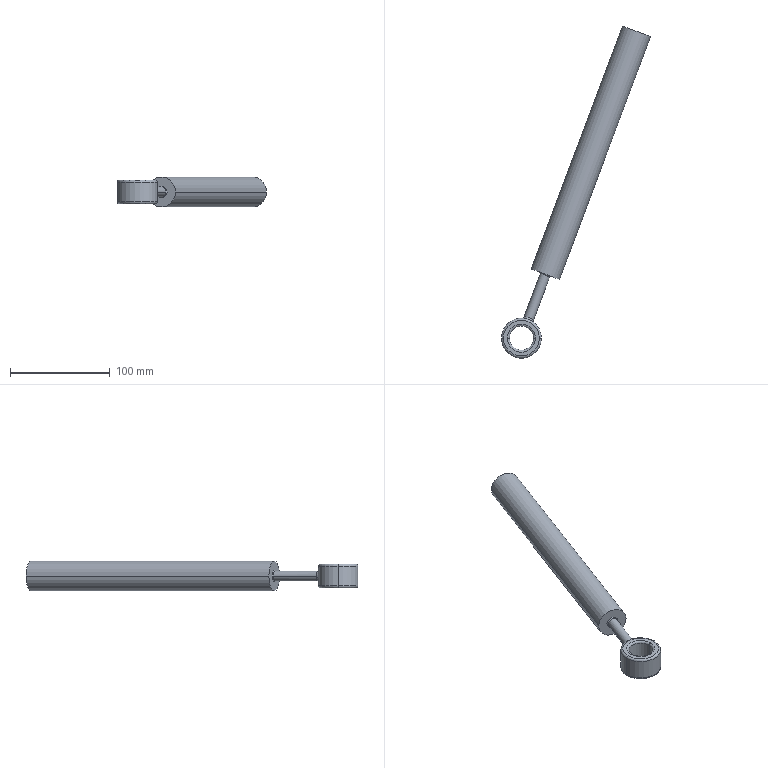Part | SolidWorks | features Fillet 2, ICE 2, Chamfer 1, Extrusion 1 | 1 solid | 24 faces | box 149.428 x 332.875 x 30.111 mm | volume 207967 mm3 | torus 8 | cylinder 8 | plane 4 | cone 2 | spline 2 | commonest cylinder face diameters 10 x2 24 x2 30.111 x2 40 x2
STEP:
#1=CARTESIAN_POINT('',(599.329,28.443,2335.07));
#2=VERTEX_POINT('',#1);
#3=CARTESIAN_POINT('',(589.965,31.954,2335.07));
#4=VERTEX_POINT('',#3);
#5=CARTESIAN_POINT('',(594.647,30.198,2335.07));
#6=DIRECTION('',(-0.3511,-0.9363,0.));
#7=DIRECTION('',(0.9363,-0.3511,0.));
#8=AXIS2_PLACEMENT_3D('',#5,#6,#7);
#9=CIRCLE('',#8,5.);
#10=EDGE_CURVE('',#2,#4,#9,.T.);
#11=ORIENTED_EDGE('',*,*,#10,.F.);
#12=CARTESIAN_POINT('',(600.616,29.028,2335.07));
#13=VERTEX_POINT('',#12);
#14=CARTESIAN_POINT('',(599.329,28.443,2335.07));
#15=DIRECTION('',(0.9103,0.4138,0.));
#16=VECTOR('',#15,1000.);
#17=LINE('',#14,#16);
#18=EDGE_CURVE('',#2,#13,#17,.T.);
#19=ORIENTED_EDGE('',*,*,#18,.T.);
#20=CARTESIAN_POINT('',(589.38,33.241,2335.07));
#21=VERTEX_POINT('',#20);
#22=CARTESIAN_POINT('',(594.998,31.135,2335.07));
#23=DIRECTION('',(0.3511,0.9363,0.));
#24=DIRECTION('',(0.9363,-0.3511,0.));
#25=AXIS2_PLACEMENT_3D('',#22,#23,#24);
#26=CIRCLE('',#25,6.);
#27=EDGE_CURVE('',#21,#13,#26,.T.);
#28=ORIENTED_EDGE('',*,*,#27,.F.);
#29=CARTESIAN_POINT('',(589.965,31.954,2335.07));
#30=DIRECTION('',(-0.4138,0.9103,0.));
#31=VECTOR('',#30,1000.);
#32=LINE('',#29,#31);
#33=EDGE_CURVE('',#4,#21,#32,.T.);
#34=ORIENTED_EDGE('',*,*,#33,.F.);
#35=EDGE_LOOP('',(#11,#19,#28,#34));
#36=FACE_OUTER_BOUND('',#35,.T.);
#37=CARTESIAN_POINT('',(594.647,30.198,2335.07));
#38=DIRECTION('',(0.3511,0.9363,0.));
#39=DIRECTION('',(-0.9363,0.3511,0.));
#40=AXIS2_PLACEMENT_3D('',#37,#38,#39);
#41=CONICAL_SURFACE('',#40,5.,0.7854);
#42=ADVANCED_FACE('',(#36),#41,.T.);
#43=CARTESIAN_POINT('',(550.949,-33.005,2345.07));
#44=VERTEX_POINT('',#43);
#45=CARTESIAN_POINT('',(590.949,-33.005,2345.07));
#46=VERTEX_POINT('',#45);
#47=CARTESIAN_POINT('',(570.949,-33.005,2345.07));
#48=DIRECTION('',(0.,0.,-1.));
#49=DIRECTION('',(1.,0.,0.));
#50=AXIS2_PLACEMENT_3D('',#47,#48,#49);
#51=CIRCLE('',#50,20.);
#52=EDGE_CURVE('',#44,#46,#51,.T.);
#53=ORIENTED_EDGE('',*,*,#52,.F.);
#54=CARTESIAN_POINT('',(552.949,-33.005,2347.07));
#55=VERTEX_POINT('',#54);
#56=CARTESIAN_POINT('',(552.949,-33.005,2345.07));
#57=DIRECTION('',(0.,1.,0.));
#58=DIRECTION('',(-1.,0.,0.));
#59=AXIS2_PLACEMENT_3D('',#56,#57,#58);
#60=CIRCLE('',#59,2.);
#61=EDGE_CURVE('',#44,#55,#60,.T.);
#62=ORIENTED_EDGE('',*,*,#61,.T.);
#63=CARTESIAN_POINT('',(588.949,-33.005,2347.07));
#64=VERTEX_POINT('',#63);
#65=CARTESIAN_POINT('',(570.949,-33.005,2347.07));
#66=DIRECTION('',(0.,0.,1.));
#67=DIRECTION('',(1.,0.,0.));
#68=AXIS2_PLACEMENT_3D('',#65,#66,#67);
#69=CIRCLE('',#68,18.);
#70=EDGE_CURVE('',#64,#55,#69,.T.);
#71=ORIENTED_EDGE('',*,*,#70,.F.);
#72=CARTESIAN_POINT('',(588.949,-33.005,2345.07));
#73=DIRECTION('',(0.,-1.,0.));
#74=DIRECTION('',(0.,0.,-1.));
#75=AXIS2_PLACEMENT_3D('',#72,#73,#74);
#76=CIRCLE('',#75,2.);
#77=EDGE_CURVE('',#46,#64,#76,.T.);
#78=ORIENTED_EDGE('',*,*,#77,.F.);
#79=EDGE_LOOP('',(#53,#62,#71,#78));
#80=FACE_OUTER_BOUND('',#79,.T.);
#81=CARTESIAN_POINT('',(570.949,-33.005,2345.07));
#82=DIRECTION('',(0.,0.,1.));
#83=DIRECTION('',(1.,0.,0.));
#84=AXIS2_PLACEMENT_3D('',#81,#82,#83);
#85=TOROIDAL_SURFACE('',#84,18.,2.);
#86=ADVANCED_FACE('',(#80),#85,.T.);
#87=CARTESIAN_POINT('',(590.949,-33.005,2325.07));
#88=VERTEX_POINT('',#87);
#89=CARTESIAN_POINT('',(550.949,-33.005,2325.07));
#90=VERTEX_POINT('',#89);
#91=CARTESIAN_POINT('',(570.949,-33.005,2325.07));
#92=DIRECTION('',(0.,0.,1.));
#93=DIRECTION('',(-1.,0.,0.));
#94=AXIS2_PLACEMENT_3D('',#91,#92,#93);
#95=CIRCLE('',#94,20.);
#96=EDGE_CURVE('',#88,#90,#95,.T.);
#97=ORIENTED_EDGE('',*,*,#96,.F.);
#98=CARTESIAN_POINT('',(588.949,-33.005,2323.07));
#99=VERTEX_POINT('',#98);
#100=CARTESIAN_POINT('',(588.949,-33.005,2325.07));
#101=DIRECTION('',(0.,1.,0.));
#102=DIRECTION('',(-1.,0.,0.));
#103=AXIS2_PLACEMENT_3D('',#100,#101,#102);
#104=CIRCLE('',#103,2.);
#105=EDGE_CURVE('',#88,#99,#104,.T.);
#106=ORIENTED_EDGE('',*,*,#105,.T.);
#107=CARTESIAN_POINT('',(552.949,-33.005,2323.07));
#108=VERTEX_POINT('',#107);
#109=CARTESIAN_POINT('',(570.949,-33.005,2323.07));
#110=DIRECTION('',(0.,0.,-1.));
#111=DIRECTION('',(-1.,0.,0.));
#112=AXIS2_PLACEMENT_3D('',#109,#110,#111);
#113=CIRCLE('',#112,18.);
#114=EDGE_CURVE('',#108,#99,#113,.T.);
#115=ORIENTED_EDGE('',*,*,#114,.F.);
#116=CARTESIAN_POINT('',(552.949,-33.005,2325.07));
#117=DIRECTION('',(0.,-1.,0.));
#118=DIRECTION('',(0.,0.,-1.));
#119=AXIS2_PLACEMENT_3D('',#116,#117,#118);
#120=CIRCLE('',#119,2.);
#121=EDGE_CURVE('',#90,#108,#120,.T.);
#122=ORIENTED_EDGE('',*,*,#121,.F.);
#123=EDGE_LOOP('',(#97,#106,#115,#122));
#124=FACE_OUTER_BOUND('',#123,.T.);
#125=CARTESIAN_POINT('',(570.949,-33.005,2325.07));
#126=DIRECTION('',(0.,0.,-1.));
#127=DIRECTION('',(-1.,0.,0.));
#128=AXIS2_PLACEMENT_3D('',#125,#126,#127);
#129=TOROIDAL_SURFACE('',#128,18.,2.);
#130=ADVANCED_FACE('',(#124),#129,.T.);
#131=CARTESIAN_POINT('',(584.949,-33.005,2323.07));
#132=VERTEX_POINT('',#131);
#133=CARTESIAN_POINT('',(556.949,-33.005,2323.07));
#134=VERTEX_POINT('',#133);
#135=CARTESIAN_POINT('',(570.949,-33.005,2323.07));
#136=DIRECTION('',(0.,0.,1.));
#137=DIRECTION('',(-1.,0.,0.));
#138=AXIS2_PLACEMENT_3D('',#135,#136,#137);
#139=CIRCLE('',#138,14.);
#140=EDGE_CURVE('',#132,#134,#139,.T.);
#141=ORIENTED_EDGE('',*,*,#140,.F.);
#142=CARTESIAN_POINT('',(582.949,-33.005,2325.07));
#143=VERTEX_POINT('',#142);
#144=CARTESIAN_POINT('',(584.949,-33.005,2325.07));
#145=DIRECTION('',(0.,1.,0.));
#146=DIRECTION('',(-1.,0.,0.));
#147=AXIS2_PLACEMENT_3D('',#144,#145,#146);
#148=CIRCLE('',#147,2.);
#149=EDGE_CURVE('',#132,#143,#148,.T.);
#150=ORIENTED_EDGE('',*,*,#149,.T.);
#151=CARTESIAN_POINT('',(558.949,-33.005,2325.07));
#152=VERTEX_POINT('',#151);
#153=CARTESIAN_POINT('',(570.949,-33.005,2325.07));
#154=DIRECTION('',(0.,0.,-1.));
#155=DIRECTION('',(-1.,0.,0.));
#156=AXIS2_PLACEMENT_3D('',#153,#154,#155);
#157=CIRCLE('',#156,12.);
#158=EDGE_CURVE('',#152,#143,#157,.T.);
#159=ORIENTED_EDGE('',*,*,#158,.F.);
#160=CARTESIAN_POINT('',(556.949,-33.005,2325.07));
#161=DIRECTION('',(0.,-1.,0.));
#162=DIRECTION('',(0.,0.,-1.));
#163=AXIS2_PLACEMENT_3D('',#160,#161,#162);
#164=CIRCLE('',#163,2.);
#165=EDGE_CURVE('',#134,#152,#164,.T.);
#166=ORIENTED_EDGE('',*,*,#165,.F.);
#167=EDGE_LOOP('',(#141,#150,#159,#166));
#168=FACE_OUTER_BOUND('',#167,.T.);
#169=CARTESIAN_POINT('',(570.949,-33.005,2325.07));
#170=DIRECTION('',(0.,0.,-1.));
#171=DIRECTION('',(-1.,0.,0.));
#172=AXIS2_PLACEMENT_3D('',#169,#170,#171);
#173=TOROIDAL_SURFACE('',#172,14.,2.);
#174=ADVANCED_FACE('',(#168),#173,.T.);
#175=CARTESIAN_POINT('',(556.949,-33.005,2347.07));
#176=VERTEX_POINT('',#175);
#177=CARTESIAN_POINT('',(584.949,-33.005,2347.07));
#178=VERTEX_POINT('',#177);
#179=CARTESIAN_POINT('',(570.949,-33.005,2347.07));
#180=DIRECTION('',(0.,0.,-1.));
#181=DIRECTION('',(1.,0.,0.));
#182=AXIS2_PLACEMENT_3D('',#179,#180,#181);
#183=CIRCLE('',#182,14.);
#184=EDGE_CURVE('',#176,#178,#183,.T.);
#185=ORIENTED_EDGE('',*,*,#184,.F.);
#186=CARTESIAN_POINT('',(558.949,-33.005,2345.07));
#187=VERTEX_POINT('',#186);
#188=CARTESIAN_POINT('',(556.949,-33.005,2345.07));
#189=DIRECTION('',(0.,1.,0.));
#190=DIRECTION('',(-1.,0.,0.));
#191=AXIS2_PLACEMENT_3D('',#188,#189,#190);
#192=CIRCLE('',#191,2.);
#193=EDGE_CURVE('',#176,#187,#192,.T.);
#194=ORIENTED_EDGE('',*,*,#193,.T.);
#195=CARTESIAN_POINT('',(582.949,-33.005,2345.07));
#196=VERTEX_POINT('',#195);
#197=CARTESIAN_POINT('',(570.949,-33.005,2345.07));
#198=DIRECTION('',(0.,0.,1.));
#199=DIRECTION('',(1.,0.,0.));
#200=AXIS2_PLACEMENT_3D('',#197,#198,#199);
#201=CIRCLE('',#200,12.);
#202=EDGE_CURVE('',#196,#187,#201,.T.);
#203=ORIENTED_EDGE('',*,*,#202,.F.);
#204=CARTESIAN_POINT('',(584.949,-33.005,2345.07));
#205=DIRECTION('',(0.,-1.,0.));
#206=DIRECTION('',(0.,0.,-1.));
#207=AXIS2_PLACEMENT_3D('',#204,#205,#206);
#208=CIRCLE('',#207,2.);
#209=EDGE_CURVE('',#178,#196,#208,.T.);
#210=ORIENTED_EDGE('',*,*,#209,.F.);
#211=EDGE_LOOP('',(#185,#194,#203,#210));
#212=FACE_OUTER_BOUND('',#211,.T.);
#213=CARTESIAN_POINT('',(570.949,-33.005,2345.07));
#214=DIRECTION('',(0.,0.,1.));
#215=DIRECTION('',(1.,0.,0.));
#216=AXIS2_PLACEMENT_3D('',#213,#214,#215);
#217=TOROIDAL_SURFACE('',#216,14.,2.);
#218=ADVANCED_FACE('',(#212),#217,.T.);
#219=CARTESIAN_POINT('',(582.785,-15.062,2336.528));
#220=VERTEX_POINT('',#219);
#221=CARTESIAN_POINT('',(582.953,-15.231,2335.07));
#222=VERTEX_POINT('',#221);
#223=CARTESIAN_POINT('',(582.785,-15.062,2336.528));
#224=CARTESIAN_POINT('',(582.84,-15.117,2336.294));
#225=CARTESIAN_POINT('',(582.882,-15.159,2336.055));
#226=CARTESIAN_POINT('',(582.939,-15.217,2335.565));
#227=CARTESIAN_POINT('',(582.953,-15.231,2335.316));
#228=CARTESIAN_POINT('',(582.953,-15.231,2335.07));
#229=B_SPLINE_CURVE_WITH_KNOTS('',3,(#223,#224,#225,#226,#227,#228),.UNSPECIFIED.,.F.,.F.,(4,2,4),(0.01457,0.01532,0.01607),.UNSPECIFIED.);
#230=EDGE_CURVE('',#220,#222,#229,.T.);
#231=ORIENTED_EDGE('',*,*,#230,.F.);
#232=CARTESIAN_POINT('',(583.337,-17.304,2337.111));
#233=VERTEX_POINT('',#232);
#234=CARTESIAN_POINT('',(584.576,-15.734,2337.111));
#235=DIRECTION('',(-0.2392,0.1887,0.9525));
#236=DIRECTION('',(0.9699,0.,0.2436));
#237=AXIS2_PLACEMENT_3D('',#234,#235,#236);
#238=CIRCLE('',#237,2.);
#239=EDGE_CURVE('',#220,#233,#238,.T.);
#240=ORIENTED_EDGE('',*,*,#239,.T.);
#241=CARTESIAN_POINT('',(571.937,-13.029,2333.032));
#242=VERTEX_POINT('',#241);
#243=CARTESIAN_POINT('',(571.937,-13.029,2333.032));
#244=CARTESIAN_POINT('',(572.061,-13.036,2332.605));
#245=CARTESIAN_POINT('',(572.221,-13.045,2332.196));
#246=CARTESIAN_POINT('',(572.514,-13.066,2331.608));
#247=CARTESIAN_POINT('',(572.621,-13.075,2331.417));
#248=CARTESIAN_POINT('',(572.852,-13.095,2331.042));
#249=CARTESIAN_POINT('',(572.977,-13.108,2330.858));
#250=CARTESIAN_POINT('',(573.374,-13.151,2330.329));
#251=CARTESIAN_POINT('',(573.668,-13.188,2330.005));
#252=CARTESIAN_POINT('',(574.312,-13.287,2329.415));
#253=CARTESIAN_POINT('',(574.667,-13.35,2329.148));
#254=CARTESIAN_POINT('',(575.406,-13.504,2328.7));
#255=CARTESIAN_POINT('',(575.794,-13.596,2328.516));
#256=CARTESIAN_POINT('',(576.606,-13.817,2328.235));
#257=CARTESIAN_POINT('',(577.019,-13.943,2328.142));
#258=CARTESIAN_POINT('',(577.637,-14.155,2328.077));
#259=CARTESIAN_POINT('',(577.844,-14.23,2328.068));
#260=CARTESIAN_POINT('',(578.257,-14.387,2328.074));
#261=CARTESIAN_POINT('',(578.464,-14.469,2328.09));
#262=CARTESIAN_POINT('',(579.067,-14.722,2328.175));
#263=CARTESIAN_POINT('',(579.453,-14.898,2328.28));
#264=CARTESIAN_POINT('',(580.009,-15.173,2328.507));
#265=CARTESIAN_POINT('',(580.191,-15.267,2328.595));
#266=CARTESIAN_POINT('',(580.541,-15.454,2328.79));
#267=CARTESIAN_POINT('',(580.709,-15.547,2328.898));
#268=CARTESIAN_POINT('',(581.191,-15.822,2329.248));
#269=CARTESIAN_POINT('',(581.486,-16.003,2329.517));
#270=CARTESIAN_POINT('',(582.028,-16.351,2330.129));
#271=CARTESIAN_POINT('',(582.267,-16.513,2330.461));
#272=CARTESIAN_POINT('',(582.58,-16.734,2330.996));
#273=CARTESIAN_POINT('',(582.678,-16.805,2331.18));
#274=CARTESIAN_POINT('',(582.858,-16.937,2331.561));
#275=CARTESIAN_POINT('',(582.942,-16.999,2331.758));
#276=CARTESIAN_POINT('',(583.166,-17.169,2332.356));
#277=CARTESIAN_POINT('',(583.285,-17.262,2332.769));
#278=CARTESIAN_POINT('',(583.462,-17.402,2333.62));
#279=CARTESIAN_POINT('',(583.52,-17.45,2334.06));
#280=CARTESIAN_POINT('',(583.574,-17.493,2334.936));
#281=CARTESIAN_POINT('',(583.57,-17.49,2335.375));
#282=CARTESIAN_POINT('',(583.5,-17.433,2336.255));
#283=CARTESIAN_POINT('',(583.434,-17.38,2336.69));
#284=CARTESIAN_POINT('',(583.337,-17.304,2337.111));
#285=B_SPLINE_CURVE_WITH_KNOTS('',3,(#243,#244,#245,#246,#247,#248,#249,#250,#251,#252,#253,#254,#255,#256,#257,#258,#259,#260,#261,#262,#263,#264,#265,#266,#267,#268,#269,#270,#271,#272,#273,#274,#275,#276,#277,#278,#279,#280,#281,#282,#283,#284),.UNSPECIFIED.,.F.,.F.,(4,2,2,2,2,2,2,2,2,2,2,2,2,2,2,2,2,2,2,2,4),(0.002059,0.003378,0.004038,0.004697,0.006016,0.007335,0.008654,0.009973,0.01063,0.01129,0.01261,0.01327,0.01393,0.01525,0.01657,0.01723,0.01789,0.01921,0.02053,0.02184,0.02316),.UNSPECIFIED.);
#286=EDGE_CURVE('',#242,#233,#285,.T.);
#287=ORIENTED_EDGE('',*,*,#286,.F.);
#288=CARTESIAN_POINT('',(573.828,-11.704,2333.614));
#289=VERTEX_POINT('',#288);
#290=CARTESIAN_POINT('',(572.036,-11.032,2333.032));
#291=DIRECTION('',(0.304,-0.01504,-0.9525));
#292=DIRECTION('',(-0.9526,0.,-0.3041));
#293=AXIS2_PLACEMENT_3D('',#290,#291,#292);
#294=CIRCLE('',#293,2.);
#295=EDGE_CURVE('',#289,#242,#294,.T.);
#296=ORIENTED_EDGE('',*,*,#295,.F.);
#297=CARTESIAN_POINT('',(582.953,-15.231,2335.07));
#298=CARTESIAN_POINT('',(582.953,-15.231,2334.771));
#299=CARTESIAN_POINT('',(582.933,-15.21,2334.473));
#300=CARTESIAN_POINT('',(582.849,-15.126,2333.879));
#301=CARTESIAN_POINT('',(582.787,-15.063,2333.59));
#302=CARTESIAN_POINT('',(582.624,-14.905,2333.036));
#303=CARTESIAN_POINT('',(582.523,-14.809,2332.768));
#304=CARTESIAN_POINT('',(582.281,-14.589,2332.259));
#305=CARTESIAN_POINT('',(582.143,-14.468,2332.021));
#306=CARTESIAN_POINT('',(581.832,-14.21,2331.579));
#307=CARTESIAN_POINT('',(581.657,-14.071,2331.373));
#308=CARTESIAN_POINT('',(581.275,-13.788,2331.002));
#309=CARTESIAN_POINT('',(581.069,-13.645,2330.838));
#310=CARTESIAN_POINT('',(580.627,-13.359,2330.553));
#311=CARTESIAN_POINT('',(580.387,-13.215,2330.431));
#312=CARTESIAN_POINT('',(579.887,-12.94,2330.24));
#313=CARTESIAN_POINT('',(579.627,-12.81,2330.17));
#314=CARTESIAN_POINT('',(579.088,-12.566,2330.081));
#315=CARTESIAN_POINT('',(578.804,-12.451,2330.063));
#316=CARTESIAN_POINT('',(578.239,-12.249,2330.082));
#317=CARTESIAN_POINT('',(577.956,-12.16,2330.119));
#318=CARTESIAN_POINT('',(577.389,-12.006,2330.245));
#319=CARTESIAN_POINT('',(577.104,-11.941,2330.335));
#320=CARTESIAN_POINT('',(576.558,-11.836,2330.561));
#321=CARTESIAN_POINT('',(576.294,-11.796,2330.697));
#322=CARTESIAN_POINT('',(575.785,-11.734,2331.015));
#323=CARTESIAN_POINT('',(575.542,-11.714,2331.196));
#324=CARTESIAN_POINT('',(575.093,-11.687,2331.592));
#325=CARTESIAN_POINT('',(574.885,-11.681,2331.808));
#326=CARTESIAN_POINT('',(574.504,-11.678,2332.279));
#327=CARTESIAN_POINT('',(574.335,-11.681,2332.529));
#328=CARTESIAN_POINT('',(574.045,-11.691,2333.052));
#329=CARTESIAN_POINT('',(573.924,-11.698,2333.326));
#330=CARTESIAN_POINT('',(573.828,-11.704,2333.614));
#331=B_SPLINE_CURVE_WITH_KNOTS('',3,(#297,#298,#299,#300,#301,#302,#303,#304,#305,#306,#307,#308,#309,#310,#311,#312,#313,#314,#315,#316,#317,#318,#319,#320,#321,#322,#323,#324,#325,#326,#327,#328,#329,#330),.UNSPECIFIED.,.F.,.F.,(4,2,2,2,2,2,2,2,2,2,2,2,2,2,2,2,4),(0.01607,0.01698,0.01789,0.0188,0.01972,0.02063,0.02154,0.02245,0.02336,0.02427,0.02518,0.02609,0.027,0.02791,0.02882,0.02974,0.03065),.UNSPECIFIED.);
#332=EDGE_CURVE('',#222,#289,#331,.T.);
#333=ORIENTED_EDGE('',*,*,#332,.F.);
#334=EDGE_LOOP('',(#231,#240,#287,#296,#333));
#335=FACE_OUTER_BOUND('',#334,.T.);
#336=CARTESIAN_POINT('',(582.785,-15.062,2336.528));
#337=CARTESIAN_POINT('',(582.229,-16.429,2336.659));
#338=CARTESIAN_POINT('',(583.337,-17.304,2337.111));
#339=CARTESIAN_POINT('',(582.859,-15.135,2336.217));
#340=CARTESIAN_POINT('',(582.324,-16.493,2336.326));
#341=CARTESIAN_POINT('',(583.437,-17.382,2336.676));
#342=CARTESIAN_POINT('',(582.91,-15.187,2335.891));
#343=CARTESIAN_POINT('',(582.391,-16.539,2335.969));
#344=CARTESIAN_POINT('',(583.505,-17.438,2336.219));
#345=CARTESIAN_POINT('',(582.96,-15.238,2335.232));
#346=CARTESIAN_POINT('',(582.457,-16.584,2335.249));
#347=CARTESIAN_POINT('',(583.573,-17.492,2335.297));
#348=CARTESIAN_POINT('',(582.959,-15.238,2334.904));
#349=CARTESIAN_POINT('',(582.456,-16.584,2334.887));
#350=CARTESIAN_POINT('',(583.573,-17.492,2334.837));
#351=CARTESIAN_POINT('',(582.909,-15.187,2334.25));
#352=CARTESIAN_POINT('',(582.391,-16.539,2334.171));
#353=CARTESIAN_POINT('',(583.505,-17.437,2333.922));
#354=CARTESIAN_POINT('',(582.859,-15.135,2333.922));
#355=CARTESIAN_POINT('',(582.324,-16.493,2333.813));
#356=CARTESIAN_POINT('',(583.437,-17.382,2333.463));
#357=CARTESIAN_POINT('',(582.709,-14.987,2333.296));
#358=CARTESIAN_POINT('',(582.132,-16.364,2333.138));
#359=CARTESIAN_POINT('',(583.236,-17.224,2332.586));
#360=CARTESIAN_POINT('',(582.611,-14.892,2332.995));
#361=CARTESIAN_POINT('',(582.006,-16.281,2332.818));
#362=CARTESIAN_POINT('',(583.104,-17.121,2332.165));
#363=CARTESIAN_POINT('',(582.427,-14.721,2332.561));
#364=CARTESIAN_POINT('',(581.777,-16.136,2332.367));
#365=CARTESIAN_POINT('',(582.857,-16.936,2331.558));
#366=CARTESIAN_POINT('',(582.359,-14.66,2332.42));
#367=CARTESIAN_POINT('',(581.693,-16.083,2332.222));
#368=CARTESIAN_POINT('',(582.767,-16.869,2331.36));
#369=CARTESIAN_POINT('',(582.214,-14.531,2332.15));
#370=CARTESIAN_POINT('',(581.516,-15.975,2331.946));
#371=CARTESIAN_POINT('',(582.573,-16.729,2330.981));
#372=CARTESIAN_POINT('',(582.136,-14.463,2332.019));
#373=CARTESIAN_POINT('',(581.422,-15.918,2331.815));
#374=CARTESIAN_POINT('',(582.469,-16.655,2330.799));
#375=CARTESIAN_POINT('',(581.969,-14.323,2331.769));
#376=CARTESIAN_POINT('',(581.225,-15.802,2331.567));
#377=CARTESIAN_POINT('',(582.247,-16.501,2330.449));
#378=CARTESIAN_POINT('',(581.88,-14.25,2331.649));
#379=CARTESIAN_POINT('',(581.121,-15.742,2331.45));
#380=CARTESIAN_POINT('',(582.129,-16.421,2330.281));
#381=CARTESIAN_POINT('',(581.69,-14.099,2331.419));
#382=CARTESIAN_POINT('',(580.904,-15.619,2331.229));
#383=CARTESIAN_POINT('',(581.878,-16.254,2329.958));
#384=CARTESIAN_POINT('',(581.589,-14.021,2331.308));
#385=CARTESIAN_POINT('',(580.79,-15.556,2331.125));
#386=CARTESIAN_POINT('',(581.745,-16.168,2329.804));
#387=CARTESIAN_POINT('',(581.273,-13.786,2330.998));
#388=CARTESIAN_POINT('',(580.439,-15.367,2330.836));
#389=CARTESIAN_POINT('',(581.328,-15.906,2329.369));
#390=CARTESIAN_POINT('',(581.045,-13.627,2330.818));
#391=CARTESIAN_POINT('',(580.195,-15.243,2330.677));
#392=CARTESIAN_POINT('',(581.029,-15.727,2329.117));
#393=CARTESIAN_POINT('',(580.551,-13.311,2330.51));
#394=CARTESIAN_POINT('',(579.691,-14.998,2330.414));
#395=CARTESIAN_POINT('',(580.385,-15.367,2328.686));
#396=CARTESIAN_POINT('',(580.281,-13.153,2330.382));
#397=CARTESIAN_POINT('',(579.428,-14.877,2330.311));
#398=CARTESIAN_POINT('',(580.035,-15.183,2328.507));
#399=CARTESIAN_POINT('',(579.723,-12.857,2330.191));
#400=CARTESIAN_POINT('',(578.903,-14.647,2330.161));
#401=CARTESIAN_POINT('',(579.315,-14.834,2328.24));
#402=CARTESIAN_POINT('',(579.433,-12.718,2330.127));
#403=CARTESIAN_POINT('',(578.641,-14.539,2330.113));
#404=CARTESIAN_POINT('',(578.942,-14.667,2328.15));
#405=CARTESIAN_POINT('',(578.98,-12.524,2330.078));
#406=CARTESIAN_POINT('',(578.239,-14.38,2330.076));
#407=CARTESIAN_POINT('',(578.362,-14.428,2328.082));
#408=CARTESIAN_POINT('',(578.825,-12.462,2330.07));
#409=CARTESIAN_POINT('',(578.104,-14.328,2330.07));
#410=CARTESIAN_POINT('',(578.164,-14.351,2328.07));
#411=CARTESIAN_POINT('',(578.516,-12.346,2330.07));
#412=CARTESIAN_POINT('',(577.834,-14.227,2330.07));
#413=CARTESIAN_POINT('',(577.771,-14.203,2328.07));
#414=CARTESIAN_POINT('',(578.361,-12.292,2330.079));
#415=CARTESIAN_POINT('',(577.699,-14.178,2330.076));
#416=CARTESIAN_POINT('',(577.574,-14.133,2328.082));
#417=CARTESIAN_POINT('',(577.895,-12.141,2330.127));
#418=CARTESIAN_POINT('',(577.295,-14.034,2330.113));
#419=CARTESIAN_POINT('',(576.984,-13.933,2328.15));
#420=CARTESIAN_POINT('',(577.582,-12.054,2330.192));
#421=CARTESIAN_POINT('',(577.023,-13.943,2330.161));
#422=CARTESIAN_POINT('',(576.589,-13.812,2328.24));
#423=CARTESIAN_POINT('',(576.961,-11.909,2330.385));
#424=CARTESIAN_POINT('',(576.472,-13.769,2330.314));
#425=CARTESIAN_POINT('',(575.809,-13.6,2328.511));
#426=CARTESIAN_POINT('',(576.661,-11.853,2330.511));
#427=CARTESIAN_POINT('',(576.2,-13.689,2330.415));
#428=CARTESIAN_POINT('',(575.434,-13.511,2328.687));
#429=CARTESIAN_POINT('',(576.08,-11.766,2330.819));
#430=CARTESIAN_POINT('',(575.658,-13.542,2330.678));
#431=CARTESIAN_POINT('',(574.711,-13.358,2329.119));
#432=CARTESIAN_POINT('',(575.798,-11.735,2331.004));
#433=CARTESIAN_POINT('',(575.387,-13.474,2330.841));
#434=CARTESIAN_POINT('',(574.36,-13.295,2329.377));
#435=CARTESIAN_POINT('',(575.277,-11.695,2331.417));
#436=CARTESIAN_POINT('',(574.874,-13.358,2331.224));
#437=CARTESIAN_POINT('',(573.716,-13.195,2329.955));
#438=CARTESIAN_POINT('',(575.037,-11.685,2331.646));
#439=CARTESIAN_POINT('',(574.63,-13.308,2331.443));
#440=CARTESIAN_POINT('',(573.42,-13.156,2330.276));
#441=CARTESIAN_POINT('',(574.707,-11.679,2332.024));
#442=CARTESIAN_POINT('',(574.288,-13.244,2331.82));
#443=CARTESIAN_POINT('',(573.015,-13.111,2330.805));
#444=CARTESIAN_POINT('',(574.603,-11.679,2332.156));
#445=CARTESIAN_POINT('',(574.178,-13.224,2331.953));
#446=CARTESIAN_POINT('',(572.886,-13.099,2330.991));
#447=CARTESIAN_POINT('',(574.408,-11.681,2332.428));
#448=CARTESIAN_POINT('',(573.974,-13.19,2332.229));
#449=CARTESIAN_POINT('',(572.648,-13.077,2331.37));
#450=CARTESIAN_POINT('',(574.318,-11.682,2332.567));
#451=CARTESIAN_POINT('',(573.878,-13.175,2332.373));
#452=CARTESIAN_POINT('',(572.537,-13.068,2331.566));
#453=CARTESIAN_POINT('',(574.07,-11.69,2332.996));
#454=CARTESIAN_POINT('',(573.613,-13.134,2332.819));
#455=CARTESIAN_POINT('',(572.233,-13.045,2332.167));
#456=CARTESIAN_POINT('',(573.933,-11.697,2333.297));
#457=CARTESIAN_POINT('',(573.463,-13.114,2333.14));
#458=CARTESIAN_POINT('',(572.066,-13.036,2332.588));
#459=CARTESIAN_POINT('',(573.828,-11.704,2333.614));
#460=CARTESIAN_POINT('',(573.347,-13.099,2333.483));
#461=CARTESIAN_POINT('',(571.937,-13.029,2333.032));
#462=(BOUNDED_SURFACE()B_SPLINE_SURFACE(3,2,((#336,#337,#338),(#339,#340,#341),(#342,#343,#344),(#345,#346,#347),(#348,#349,#350),(#351,#352,#353),(#354,#355,#356),(#357,#358,#359),(#360,#361,#362),(#363,#364,#365),(#366,#367,#368),(#369,#370,#371),(#372,#373,#374),(#375,#376,#377),(#378,#379,#380),(#381,#382,#383),(#384,#385,#386),(#387,#388,#389),(#390,#391,#392),(#393,#394,#395),(#396,#397,#398),(#399,#400,#401),(#402,#403,#404),(#405,#406,#407),(#408,#409,#410),(#411,#412,#413),(#414,#415,#416),(#417,#418,#419),(#420,#421,#422),(#423,#424,#425),(#426,#427,#428),(#429,#430,#431),(#432,#433,#434),(#435,#436,#437),(#438,#439,#440),(#441,#442,#443),(#444,#445,#446),(#447,#448,#449),(#450,#451,#452),(#453,#454,#455),(#456,#457,#458),(#459,#460,#461)),.UNSPECIFIED.,.F.,.F.,.T.)B_SPLINE_SURFACE_WITH_KNOTS((4,2,2,2,2,2,2,2,2,2,2,2,2,2,2,2,2,2,2,2,4),(3,3),(0.022,0.02338,0.02475,0.02613,0.02751,0.02819,0.02888,0.02957,0.03026,0.03163,0.03301,0.03438,0.03507,0.03576,0.03713,0.03851,0.03988,0.04126,0.04195,0.04263,0.04401),(0.,1.),.UNSPECIFIED.)GEOMETRIC_REPRESENTATION_ITEM()RATIONAL_B_SPLINE_SURFACE(((1.,0.8035,1.),(1.,0.8071,1.),(1.,0.8096,1.),(1.,0.8122,1.),(1.,0.8122,1.),(1.,0.8096,1.),(1.,0.8071,1.),(1.,0.7998,1.),(1.,0.7951,1.),(1.,0.7869,1.),(1.,0.7839,1.),(1.,0.7778,1.),(1.,0.7746,1.),(1.,0.768,1.),(1.,0.7647,1.),(1.,0.7579,1.),(1.,0.7544,1.),(1.,0.7442,1.),(1.,0.7377,1.),(1.,0.7259,1.),(1.,0.7206,1.),(1.,0.7125,1.),(1.,0.7097,1.),(1.,0.7075,1.),(1.,0.7071,1.),(1.,0.7071,1.),(1.,0.7075,1.),(1.,0.7097,1.),(1.,0.7125,1.),(1.,0.7207,1.),(1.,0.7259,1.),(1.,0.7377,1.),(1.,0.7444,1.),(1.,0.7579,1.),(1.,0.7648,1.),(1.,0.7747,1.),(1.,0.7779,1.),(1.,0.7841,1.),(1.,0.787,1.),(1.,0.7952,1.),(1.,0.7998,1.),(1.,0.8035,1.)))REPRESENTATION_ITEM('')SURFACE());
#463=ADVANCED_FACE('',(#335),#462,.F.);
#464=CARTESIAN_POINT('',(570.949,-33.005,2345.07));
#465=DIRECTION('',(0.,0.,1.));
#466=DIRECTION('',(1.,0.,0.));
#467=AXIS2_PLACEMENT_3D('',#464,#465,#466);
#468=CIRCLE('',#467,12.);
#469=EDGE_CURVE('',#187,#196,#468,.T.);
#470=ORIENTED_EDGE('',*,*,#469,.T.);
#471=CARTESIAN_POINT('',(582.949,-33.005,2403.639));
#472=DIRECTION('',(0.,0.,-1.));
#473=VECTOR('',#472,1000.);
#474=LINE('',#471,#473);
#475=EDGE_CURVE('',#196,#143,#474,.T.);
#476=ORIENTED_EDGE('',*,*,#475,.T.);
#477=CARTESIAN_POINT('',(570.949,-33.005,2325.07));
#478=DIRECTION('',(0.,0.,-1.));
#479=DIRECTION('',(-1.,0.,0.));
#480=AXIS2_PLACEMENT_3D('',#477,#478,#479);
#481=CIRCLE('',#480,12.);
#482=EDGE_CURVE('',#143,#152,#481,.T.);
#483=ORIENTED_EDGE('',*,*,#482,.T.);
#484=CARTESIAN_POINT('',(558.949,-33.005,2403.639));
#485=DIRECTION('',(0.,0.,-1.));
#486=VECTOR('',#485,1000.);
#487=LINE('',#484,#486);
#488=EDGE_CURVE('',#187,#152,#487,.T.);
#489=ORIENTED_EDGE('',*,*,#488,.F.);
#490=EDGE_LOOP('',(#470,#476,#483,#489));
#491=FACE_OUTER_BOUND('',#490,.T.);
#492=CARTESIAN_POINT('',(570.949,-33.005,2403.639));
#493=DIRECTION('',(0.,0.,-1.));
#494=DIRECTION('',(-1.,0.,0.));
#495=AXIS2_PLACEMENT_3D('',#492,#493,#494);
#496=CYLINDRICAL_SURFACE('',#495,12.);
#497=ADVANCED_FACE('',(#491),#496,.F.);
#498=ORIENTED_EDGE('',*,*,#286,.T.);
#499=CARTESIAN_POINT('',(583.337,-17.304,2337.111));
#500=CARTESIAN_POINT('',(583.241,-17.228,2337.531));
#501=CARTESIAN_POINT('',(583.114,-17.129,2337.944));
#502=CARTESIAN_POINT('',(582.798,-16.891,2338.735));
#503=CARTESIAN_POINT('',(582.611,-16.755,2339.108));
#504=CARTESIAN_POINT('',(582.286,-16.528,2339.633));
#505=CARTESIAN_POINT('',(582.17,-16.449,2339.802));
#506=CARTESIAN_POINT('',(581.922,-16.283,2340.129));
#507=CARTESIAN_POINT('',(581.79,-16.197,2340.285));
#508=CARTESIAN_POINT('',(581.376,-15.935,2340.728));
#509=CARTESIAN_POINT('',(581.075,-15.753,2340.989));
#510=CARTESIAN_POINT('',(580.579,-15.475,2341.327));
#511=CARTESIAN_POINT('',(580.405,-15.38,2341.431));
#512=CARTESIAN_POINT('',(580.05,-15.194,2341.615));
#513=CARTESIAN_POINT('',(579.868,-15.102,2341.695));
#514=CARTESIAN_POINT('',(579.494,-14.921,2341.834));
#515=CARTESIAN_POINT('',(579.303,-14.832,2341.892));
#516=CARTESIAN_POINT('',(578.91,-14.656,2341.985));
#517=CARTESIAN_POINT('',(578.707,-14.57,2342.02));
#518=CARTESIAN_POINT('',(578.096,-14.32,2342.086));
#519=CARTESIAN_POINT('',(577.686,-14.169,2342.079));
#520=CARTESIAN_POINT('',(576.861,-13.894,2341.967));
#521=CARTESIAN_POINT('',(576.442,-13.77,2341.859));
#522=CARTESIAN_POINT('',(575.647,-13.56,2341.558));
#523=CARTESIAN_POINT('',(575.265,-13.473,2341.365));
#524=CARTESIAN_POINT('',(574.714,-13.362,2341.012));
#525=CARTESIAN_POINT('',(574.535,-13.328,2340.884));
#526=CARTESIAN_POINT('',(574.193,-13.269,2340.614));
#527=CARTESIAN_POINT('',(574.029,-13.243,2340.471));
#528=CARTESIAN_POINT('',(573.715,-13.197,2340.169));
#529=CARTESIAN_POINT('',(573.565,-13.176,2340.011));
#530=CARTESIAN_POINT('',(573.278,-13.14,2339.679));
#531=CARTESIAN_POINT('',(573.14,-13.125,2339.505));
#532=CARTESIAN_POINT('',(572.755,-13.085,2338.967));
#533=CARTESIAN_POINT('',(572.534,-13.067,2338.588));
#534=CARTESIAN_POINT('',(572.159,-13.041,2337.794));
#535=CARTESIAN_POINT('',(572.006,-13.033,2337.374));
#536=CARTESIAN_POINT('',(571.78,-13.022,2336.525));
#537=CARTESIAN_POINT('',(571.706,-13.019,2336.092));
#538=CARTESIAN_POINT('',(571.635,-13.017,2335.212));
#539=CARTESIAN_POINT('',(571.64,-13.017,2334.765));
#540=CARTESIAN_POINT('',(571.73,-13.02,2333.89));
#541=CARTESIAN_POINT('',(571.814,-13.023,2333.458));
#542=CARTESIAN_POINT('',(571.937,-13.029,2333.032));
#543=B_SPLINE_CURVE_WITH_KNOTS('',3,(#499,#500,#501,#502,#503,#504,#505,#506,#507,#508,#509,#510,#511,#512,#513,#514,#515,#516,#517,#518,#519,#520,#521,#522,#523,#524,#525,#526,#527,#528,#529,#530,#531,#532,#533,#534,#535,#536,#537,#538,#539,#540,#541,#542),.UNSPECIFIED.,.F.,.F.,(4,2,2,2,2,2,2,2,2,2,2,2,2,2,2,2,2,2,2,2,2,4),(0.02316,0.02448,0.0258,0.02646,0.02712,0.02844,0.0291,0.02976,0.03042,0.03107,0.03239,0.03371,0.03503,0.03569,0.03635,0.03701,0.03767,0.03899,0.0403,0.04162,0.04294,0.04426),.UNSPECIFIED.);
#544=EDGE_CURVE('',#233,#242,#543,.T.);
#545=ORIENTED_EDGE('',*,*,#544,.T.);
#546=EDGE_LOOP('',(#498,#545));
#547=FACE_BOUND('',#546,.T.);
#548=ORIENTED_EDGE('',*,*,#52,.T.);
#549=CARTESIAN_POINT('',(590.949,-33.005,2403.639));
#550=DIRECTION('',(0.,0.,-1.));
#551=VECTOR('',#550,1000.);
#552=LINE('',#549,#551);
#553=EDGE_CURVE('',#46,#88,#552,.T.);
#554=ORIENTED_EDGE('',*,*,#553,.T.);
#555=ORIENTED_EDGE('',*,*,#96,.T.);
#556=CARTESIAN_POINT('',(550.949,-33.005,2403.639));
#557=DIRECTION('',(0.,0.,-1.));
#558=VECTOR('',#557,1000.);
#559=LINE('',#556,#558);
#560=EDGE_CURVE('',#44,#90,#559,.T.);
#561=ORIENTED_EDGE('',*,*,#560,.F.);
#562=EDGE_LOOP('',(#548,#554,#555,#561));
#563=FACE_OUTER_BOUND('',#562,.T.);
#564=CARTESIAN_POINT('',(570.949,-33.005,2403.639));
#565=DIRECTION('',(0.,0.,-1.));
#566=DIRECTION('',(-1.,0.,0.));
#567=AXIS2_PLACEMENT_3D('',#564,#565,#566);
#568=CYLINDRICAL_SURFACE('',#567,20.);
#569=ADVANCED_FACE('',(#547,#563),#568,.T.);
#570=CARTESIAN_POINT('',(573.59,-11.721,2335.07));
#571=VERTEX_POINT('',#570);
#572=CARTESIAN_POINT('',(573.59,-11.721,2335.07));
#573=CARTESIAN_POINT('',(573.59,-11.721,2335.374));
#574=CARTESIAN_POINT('',(573.62,-11.718,2335.675));
#575=CARTESIAN_POINT('',(573.738,-11.709,2336.262));
#576=CARTESIAN_POINT('',(573.825,-11.703,2336.549));
#577=CARTESIAN_POINT('',(574.055,-11.691,2337.11));
#578=CARTESIAN_POINT('',(574.195,-11.685,2337.376));
#579=CARTESIAN_POINT('',(574.518,-11.679,2337.88));
#580=CARTESIAN_POINT('',(574.703,-11.678,2338.12));
#581=CARTESIAN_POINT('',(575.111,-11.688,2338.566));
#582=CARTESIAN_POINT('',(575.331,-11.699,2338.769));
#583=CARTESIAN_POINT('',(575.801,-11.736,2339.137));
#584=CARTESIAN_POINT('',(576.055,-11.764,2339.304));
#585=CARTESIAN_POINT('',(576.579,-11.84,2339.59));
#586=CARTESIAN_POINT('',(576.849,-11.888,2339.709));
#587=CARTESIAN_POINT('',(577.403,-12.009,2339.9));
#588=CARTESIAN_POINT('',(577.69,-12.084,2339.972));
#589=CARTESIAN_POINT('',(578.26,-12.256,2340.06));
#590=CARTESIAN_POINT('',(578.542,-12.353,2340.077));
#591=CARTESIAN_POINT('',(579.1,-12.571,2340.058));
#592=CARTESIAN_POINT('',(579.378,-12.693,2340.021));
#593=CARTESIAN_POINT('',(579.906,-12.95,2339.895));
#594=CARTESIAN_POINT('',(580.158,-13.085,2339.807));
#595=CARTESIAN_POINT('',(580.64,-13.366,2339.58));
#596=CARTESIAN_POINT('',(580.869,-13.512,2339.442));
#597=CARTESIAN_POINT('',(581.29,-13.798,2339.126));
#598=CARTESIAN_POINT('',(581.484,-13.941,2338.947));
#599=CARTESIAN_POINT('',(581.843,-14.218,2338.548));
#600=CARTESIAN_POINT('',(582.005,-14.351,2338.329));
#601=CARTESIAN_POINT('',(582.29,-14.597,2337.864));
#602=CARTESIAN_POINT('',(582.415,-14.71,2337.616));
#603=CARTESIAN_POINT('',(582.63,-14.911,2337.087));
#604=CARTESIAN_POINT('',(582.718,-14.995,2336.811));
#605=CARTESIAN_POINT('',(582.785,-15.062,2336.528));
#606=B_SPLINE_CURVE_WITH_KNOTS('',3,(#572,#573,#574,#575,#576,#577,#578,#579,#580,#581,#582,#583,#584,#585,#586,#587,#588,#589,#590,#591,#592,#593,#594,#595,#596,#597,#598,#599,#600,#601,#602,#603,#604,#605),.UNSPECIFIED.,.F.,.F.,(4,2,2,2,2,2,2,2,2,2,2,2,2,2,2,2,4),(0.,0.0009109,0.001822,0.002733,0.003643,0.004554,0.005465,0.006376,0.007287,0.008198,0.009109,0.01002,0.01093,0.01184,0.01275,0.01366,0.01457),.UNSPECIFIED.);
#607=EDGE_CURVE('',#571,#220,#606,.T.);
#608=ORIENTED_EDGE('',*,*,#607,.T.);
#609=ORIENTED_EDGE('',*,*,#230,.T.);
#610=CARTESIAN_POINT('',(566.591,-58.871,2335.07));
#611=DIRECTION('',(0.3511,0.9363,0.));
#612=VECTOR('',#611,1000.);
#613=LINE('',#610,#612);
#614=EDGE_CURVE('',#222,#2,#613,.T.);
#615=ORIENTED_EDGE('',*,*,#614,.T.);
#616=ORIENTED_EDGE('',*,*,#10,.T.);
#617=CARTESIAN_POINT('',(557.227,-55.36,2335.07));
#618=DIRECTION('',(0.3511,0.9363,0.));
#619=VECTOR('',#618,1000.);
#620=LINE('',#617,#619);
#621=EDGE_CURVE('',#571,#4,#620,.T.);
#622=ORIENTED_EDGE('',*,*,#621,.F.);
#623=EDGE_LOOP('',(#608,#609,#615,#616,#622));
#624=FACE_OUTER_BOUND('',#623,.T.);
#625=CARTESIAN_POINT('',(561.909,-57.116,2335.07));
#626=DIRECTION('',(0.3511,0.9363,0.));
#627=DIRECTION('',(-0.9363,0.3511,0.));
#628=AXIS2_PLACEMENT_3D('',#625,#626,#627);
#629=CYLINDRICAL_SURFACE('',#628,5.);
#630=ADVANCED_FACE('',(#624),#629,.T.);
#631=CARTESIAN_POINT('',(672.182,279.87,2335.07));
#632=VERTEX_POINT('',#631);
#633=CARTESIAN_POINT('',(700.377,269.299,2335.07));
#634=VERTEX_POINT('',#633);
#635=CARTESIAN_POINT('',(686.279,274.584,2335.07));
#636=DIRECTION('',(0.3511,0.9363,0.));
#637=DIRECTION('',(0.,0.,1.));
#638=AXIS2_PLACEMENT_3D('',#635,#636,#637);
#639=CIRCLE('',#638,15.056);
#640=EDGE_CURVE('',#632,#634,#639,.T.);
#641=ORIENTED_EDGE('',*,*,#640,.F.);
#642=CARTESIAN_POINT('',(580.901,36.42,2335.07));
#643=VERTEX_POINT('',#642);
#644=CARTESIAN_POINT('',(687.132,319.743,2335.07));
#645=DIRECTION('',(-0.3511,-0.9363,0.));
#646=VECTOR('',#645,1000.);
#647=LINE('',#644,#646);
#648=EDGE_CURVE('',#632,#643,#647,.T.);
#649=ORIENTED_EDGE('',*,*,#648,.T.);
#650=CARTESIAN_POINT('',(609.096,25.849,2335.07));
#651=VERTEX_POINT('',#650);
#652=CARTESIAN_POINT('',(594.998,31.135,2335.07));
#653=DIRECTION('',(-0.3511,-0.9363,0.));
#654=DIRECTION('',(0.9363,-0.3511,0.));
#655=AXIS2_PLACEMENT_3D('',#652,#653,#654);
#656=CIRCLE('',#655,15.056);
#657=EDGE_CURVE('',#651,#643,#656,.T.);
#658=ORIENTED_EDGE('',*,*,#657,.F.);
#659=CARTESIAN_POINT('',(715.327,309.172,2335.07));
#660=DIRECTION('',(-0.3511,-0.9363,0.));
#661=VECTOR('',#660,1000.);
#662=LINE('',#659,#661);
#663=EDGE_CURVE('',#634,#651,#662,.T.);
#664=ORIENTED_EDGE('',*,*,#663,.F.);
#665=EDGE_LOOP('',(#641,#649,#658,#664));
#666=FACE_OUTER_BOUND('',#665,.T.);
#667=CARTESIAN_POINT('',(701.23,314.458,2335.07));
#668=DIRECTION('',(-0.3511,-0.9363,0.));
#669=DIRECTION('',(0.9363,-0.3511,0.));
#670=AXIS2_PLACEMENT_3D('',#667,#668,#669);
#671=CYLINDRICAL_SURFACE('',#670,15.056);
#672=ADVANCED_FACE('',(#666),#671,.T.);
#673=CARTESIAN_POINT('',(686.279,274.584,2335.07));
#674=DIRECTION('',(0.3511,0.9363,0.));
#675=DIRECTION('',(0.,0.,1.));
#676=AXIS2_PLACEMENT_3D('',#673,#674,#675);
#677=CIRCLE('',#676,15.056);
#678=EDGE_CURVE('',#634,#632,#677,.T.);
#679=ORIENTED_EDGE('',*,*,#678,.T.);
#680=ORIENTED_EDGE('',*,*,#640,.T.);
#681=EDGE_LOOP('',(#679,#680));
#682=FACE_OUTER_BOUND('',#681,.T.);
#683=CARTESIAN_POINT('',(686.279,274.584,2335.07));
#684=DIRECTION('',(0.3511,0.9363,0.));
#685=DIRECTION('',(0.,0.,1.));
#686=AXIS2_PLACEMENT_3D('',#683,#684,#685);
#687=PLANE('',#686);
#688=ADVANCED_FACE('',(#682),#687,.T.);
#689=ORIENTED_EDGE('',*,*,#27,.T.);
#690=CARTESIAN_POINT('',(594.998,31.135,2335.07));
#691=DIRECTION('',(0.3511,0.9363,0.));
#692=DIRECTION('',(0.9363,-0.3511,0.));
#693=AXIS2_PLACEMENT_3D('',#690,#691,#692);
#694=CIRCLE('',#693,6.);
#695=EDGE_CURVE('',#13,#21,#694,.T.);
#696=ORIENTED_EDGE('',*,*,#695,.T.);
#697=EDGE_LOOP('',(#689,#696));
#698=FACE_BOUND('',#697,.T.);
#699=ORIENTED_EDGE('',*,*,#657,.T.);
#700=CARTESIAN_POINT('',(594.998,31.135,2335.07));
#701=DIRECTION('',(-0.3511,-0.9363,0.));
#702=DIRECTION('',(0.9363,-0.3511,0.));
#703=AXIS2_PLACEMENT_3D('',#700,#701,#702);
#704=CIRCLE('',#703,15.056);
#705=EDGE_CURVE('',#643,#651,#704,.T.);
#706=ORIENTED_EDGE('',*,*,#705,.T.);
#707=EDGE_LOOP('',(#699,#706));
#708=FACE_OUTER_BOUND('',#707,.T.);
#709=CARTESIAN_POINT('',(594.998,31.135,2335.07));
#710=DIRECTION('',(-0.3511,-0.9363,0.));
#711=DIRECTION('',(0.9363,-0.3511,0.));
#712=AXIS2_PLACEMENT_3D('',#709,#710,#711);
#713=PLANE('',#712);
#714=ADVANCED_FACE('',(#698,#708),#713,.T.);
#715=ORIENTED_EDGE('',*,*,#648,.F.);
#716=ORIENTED_EDGE('',*,*,#678,.F.);
#717=ORIENTED_EDGE('',*,*,#663,.T.);
#718=ORIENTED_EDGE('',*,*,#705,.F.);
#719=EDGE_LOOP('',(#715,#716,#717,#718));
#720=FACE_OUTER_BOUND('',#719,.T.);
#721=CARTESIAN_POINT('',(701.23,314.458,2335.07));
#722=DIRECTION('',(-0.3511,-0.9363,0.));
#723=DIRECTION('',(0.9363,-0.3511,0.));
#724=AXIS2_PLACEMENT_3D('',#721,#722,#723);
#725=CYLINDRICAL_SURFACE('',#724,15.056);
#726=ADVANCED_FACE('',(#720),#725,.T.);
#727=ORIENTED_EDGE('',*,*,#614,.F.);
#728=ORIENTED_EDGE('',*,*,#332,.T.);
#729=CARTESIAN_POINT('',(573.828,-11.704,2333.614));
#730=CARTESIAN_POINT('',(573.749,-11.708,2333.85));
#731=CARTESIAN_POINT('',(573.69,-11.713,2334.09));
#732=CARTESIAN_POINT('',(573.61,-11.719,2334.575));
#733=CARTESIAN_POINT('',(573.59,-11.721,2334.821));
#734=CARTESIAN_POINT('',(573.59,-11.721,2335.07));
#735=B_SPLINE_CURVE_WITH_KNOTS('',3,(#729,#730,#731,#732,#733,#734),.UNSPECIFIED.,.F.,.F.,(4,2,4),(0.03065,0.03139,0.03214),.UNSPECIFIED.);
#736=EDGE_CURVE('',#289,#571,#735,.T.);
#737=ORIENTED_EDGE('',*,*,#736,.T.);
#738=ORIENTED_EDGE('',*,*,#621,.T.);
#739=CARTESIAN_POINT('',(594.647,30.198,2335.07));
#740=DIRECTION('',(-0.3511,-0.9363,0.));
#741=DIRECTION('',(0.9363,-0.3511,0.));
#742=AXIS2_PLACEMENT_3D('',#739,#740,#741);
#743=CIRCLE('',#742,5.);
#744=EDGE_CURVE('',#4,#2,#743,.T.);
#745=ORIENTED_EDGE('',*,*,#744,.T.);
#746=EDGE_LOOP('',(#727,#728,#737,#738,#745));
#747=FACE_OUTER_BOUND('',#746,.T.);
#748=CARTESIAN_POINT('',(561.909,-57.116,2335.07));
#749=DIRECTION('',(0.3511,0.9363,0.));
#750=DIRECTION('',(-0.9363,0.3511,0.));
#751=AXIS2_PLACEMENT_3D('',#748,#749,#750);
#752=CYLINDRICAL_SURFACE('',#751,5.);
#753=ADVANCED_FACE('',(#747),#752,.T.);
#754=ORIENTED_EDGE('',*,*,#553,.F.);
#755=CARTESIAN_POINT('',(570.949,-33.005,2345.07));
#756=DIRECTION('',(0.,0.,-1.));
#757=DIRECTION('',(1.,0.,0.));
#758=AXIS2_PLACEMENT_3D('',#755,#756,#757);
#759=CIRCLE('',#758,20.);
#760=EDGE_CURVE('',#46,#44,#759,.T.);
#761=ORIENTED_EDGE('',*,*,#760,.T.);
#762=ORIENTED_EDGE('',*,*,#560,.T.);
#763=CARTESIAN_POINT('',(570.949,-33.005,2325.07));
#764=DIRECTION('',(0.,0.,1.));
#765=DIRECTION('',(-1.,0.,0.));
#766=AXIS2_PLACEMENT_3D('',#763,#764,#765);
#767=CIRCLE('',#766,20.);
#768=EDGE_CURVE('',#90,#88,#767,.T.);
#769=ORIENTED_EDGE('',*,*,#768,.T.);
#770=EDGE_LOOP('',(#754,#761,#762,#769));
#771=FACE_OUTER_BOUND('',#770,.T.);
#772=CARTESIAN_POINT('',(570.949,-33.005,2403.639));
#773=DIRECTION('',(0.,0.,-1.));
#774=DIRECTION('',(-1.,0.,0.));
#775=AXIS2_PLACEMENT_3D('',#772,#773,#774);
#776=CYLINDRICAL_SURFACE('',#775,20.);
#777=ADVANCED_FACE('',(#771),#776,.T.);
#778=ORIENTED_EDGE('',*,*,#475,.F.);
#779=ORIENTED_EDGE('',*,*,#202,.T.);
#780=ORIENTED_EDGE('',*,*,#488,.T.);
#781=ORIENTED_EDGE('',*,*,#158,.T.);
#782=EDGE_LOOP('',(#778,#779,#780,#781));
#783=FACE_OUTER_BOUND('',#782,.T.);
#784=CARTESIAN_POINT('',(570.949,-33.005,2403.639));
#785=DIRECTION('',(0.,0.,-1.));
#786=DIRECTION('',(-1.,0.,0.));
#787=AXIS2_PLACEMENT_3D('',#784,#785,#786);
#788=CYLINDRICAL_SURFACE('',#787,12.);
#789=ADVANCED_FACE('',(#783),#788,.F.);
#790=CARTESIAN_POINT('',(570.949,-33.005,2323.07));
#791=DIRECTION('',(0.,0.,1.));
#792=DIRECTION('',(-1.,0.,0.));
#793=AXIS2_PLACEMENT_3D('',#790,#791,#792);
#794=CIRCLE('',#793,14.);
#795=EDGE_CURVE('',#134,#132,#794,.T.);
#796=ORIENTED_EDGE('',*,*,#795,.T.);
#797=ORIENTED_EDGE('',*,*,#140,.T.);
#798=EDGE_LOOP('',(#796,#797));
#799=FACE_BOUND('',#798,.T.);
#800=ORIENTED_EDGE('',*,*,#114,.T.);
#801=CARTESIAN_POINT('',(570.949,-33.005,2323.07));
#802=DIRECTION('',(0.,0.,-1.));
#803=DIRECTION('',(-1.,0.,0.));
#804=AXIS2_PLACEMENT_3D('',#801,#802,#803);
#805=CIRCLE('',#804,18.);
#806=EDGE_CURVE('',#99,#108,#805,.T.);
#807=ORIENTED_EDGE('',*,*,#806,.T.);
#808=EDGE_LOOP('',(#800,#807));
#809=FACE_OUTER_BOUND('',#808,.T.);
#810=CARTESIAN_POINT('',(570.949,-33.005,2323.07));
#811=DIRECTION('',(0.,0.,-1.));
#812=DIRECTION('',(-1.,0.,0.));
#813=AXIS2_PLACEMENT_3D('',#810,#811,#812);
#814=PLANE('',#813);
#815=ADVANCED_FACE('',(#799,#809),#814,.T.);
#816=CARTESIAN_POINT('',(570.949,-33.005,2347.07));
#817=DIRECTION('',(0.,0.,-1.));
#818=DIRECTION('',(1.,0.,0.));
#819=AXIS2_PLACEMENT_3D('',#816,#817,#818);
#820=CIRCLE('',#819,14.);
#821=EDGE_CURVE('',#178,#176,#820,.T.);
#822=ORIENTED_EDGE('',*,*,#821,.T.);
#823=ORIENTED_EDGE('',*,*,#184,.T.);
#824=EDGE_LOOP('',(#822,#823));
#825=FACE_BOUND('',#824,.T.);
#826=ORIENTED_EDGE('',*,*,#70,.T.);
#827=CARTESIAN_POINT('',(570.949,-33.005,2347.07));
#828=DIRECTION('',(0.,0.,1.));
#829=DIRECTION('',(1.,0.,0.));
#830=AXIS2_PLACEMENT_3D('',#827,#828,#829);
#831=CIRCLE('',#830,18.);
#832=EDGE_CURVE('',#55,#64,#831,.T.);
#833=ORIENTED_EDGE('',*,*,#832,.T.);
#834=EDGE_LOOP('',(#826,#833));
#835=FACE_OUTER_BOUND('',#834,.T.);
#836=CARTESIAN_POINT('',(577.444,-15.683,2347.07));
#837=DIRECTION('',(0.,0.,1.));
#838=DIRECTION('',(0.9363,-0.3511,0.));
#839=AXIS2_PLACEMENT_3D('',#836,#837,#838);
#840=PLANE('',#839);
#841=ADVANCED_FACE('',(#825,#835),#840,.T.);
#842=ORIENTED_EDGE('',*,*,#239,.F.);
#843=ORIENTED_EDGE('',*,*,#607,.F.);
#844=ORIENTED_EDGE('',*,*,#736,.F.);
#845=ORIENTED_EDGE('',*,*,#295,.T.);
#846=ORIENTED_EDGE('',*,*,#544,.F.);
#847=EDGE_LOOP('',(#842,#843,#844,#845,#846));
#848=FACE_OUTER_BOUND('',#847,.T.);
#849=CARTESIAN_POINT('',(573.828,-11.704,2333.614));
#850=CARTESIAN_POINT('',(573.347,-13.099,2333.483));
#851=CARTESIAN_POINT('',(571.937,-13.029,2333.032));
#852=CARTESIAN_POINT('',(573.722,-11.71,2333.931));
#853=CARTESIAN_POINT('',(573.232,-13.084,2333.822));
#854=CARTESIAN_POINT('',(571.809,-13.023,2333.475));
#855=CARTESIAN_POINT('',(573.652,-11.716,2334.252));
#856=CARTESIAN_POINT('',(573.154,-13.075,2334.174));
#857=CARTESIAN_POINT('',(571.723,-13.02,2333.925));
#858=CARTESIAN_POINT('',(573.599,-11.72,2334.741));
#859=CARTESIAN_POINT('',(573.095,-13.069,2334.709));
#860=CARTESIAN_POINT('',(571.658,-13.018,2334.609));
#861=CARTESIAN_POINT('',(573.59,-11.721,2334.905));
#862=CARTESIAN_POINT('',(573.085,-13.067,2334.889));
#863=CARTESIAN_POINT('',(571.647,-13.017,2334.839));
#864=CARTESIAN_POINT('',(573.59,-11.721,2335.235));
#865=CARTESIAN_POINT('',(573.085,-13.067,2335.251));
#866=CARTESIAN_POINT('',(571.647,-13.017,2335.301));
#867=CARTESIAN_POINT('',(573.599,-11.72,2335.402));
#868=CARTESIAN_POINT('',(573.095,-13.069,2335.434));
#869=CARTESIAN_POINT('',(571.658,-13.018,2335.535));
#870=CARTESIAN_POINT('',(573.653,-11.716,2335.894));
#871=CARTESIAN_POINT('',(573.155,-13.075,2335.973));
#872=CARTESIAN_POINT('',(571.724,-13.02,2336.224));
#873=CARTESIAN_POINT('',(573.724,-11.71,2336.215));
#874=CARTESIAN_POINT('',(573.234,-13.085,2336.324));
#875=CARTESIAN_POINT('',(571.811,-13.023,2336.673));
#876=CARTESIAN_POINT('',(573.881,-11.7,2336.686));
#877=CARTESIAN_POINT('',(573.406,-13.107,2336.83));
#878=CARTESIAN_POINT('',(572.002,-13.033,2337.332));
#879=CARTESIAN_POINT('',(573.942,-11.697,2336.842));
#880=CARTESIAN_POINT('',(573.472,-13.116,2336.997));
#881=CARTESIAN_POINT('',(572.077,-13.037,2337.55));
#882=CARTESIAN_POINT('',(574.08,-11.69,2337.145));
#883=CARTESIAN_POINT('',(573.622,-13.136,2337.319));
#884=CARTESIAN_POINT('',(572.245,-13.047,2337.975));
#885=CARTESIAN_POINT('',(574.156,-11.687,2337.293));
#886=CARTESIAN_POINT('',(573.704,-13.148,2337.474));
#887=CARTESIAN_POINT('',(572.338,-13.053,2338.182));
#888=CARTESIAN_POINT('',(574.405,-11.68,2337.722));
#889=CARTESIAN_POINT('',(573.972,-13.189,2337.924));
#890=CARTESIAN_POINT('',(572.643,-13.076,2338.783));
#891=CARTESIAN_POINT('',(574.599,-11.677,2337.993));
#892=CARTESIAN_POINT('',(574.178,-13.223,2338.2));
#893=CARTESIAN_POINT('',(572.882,-13.097,2339.162));
#894=CARTESIAN_POINT('',(575.041,-11.685,2338.5));
#895=CARTESIAN_POINT('',(574.635,-13.309,2338.702));
#896=CARTESIAN_POINT('',(573.425,-13.157,2339.871));
#897=CARTESIAN_POINT('',(575.283,-11.695,2338.728));
#898=CARTESIAN_POINT('',(574.879,-13.359,2338.921));
#899=CARTESIAN_POINT('',(573.723,-13.196,2340.192));
#900=CARTESIAN_POINT('',(575.672,-11.726,2339.037));
#901=CARTESIAN_POINT('',(575.262,-13.446,2339.205));
#902=CARTESIAN_POINT('',(574.205,-13.271,2340.624));
#903=CARTESIAN_POINT('',(575.807,-11.738,2339.134));
#904=CARTESIAN_POINT('',(575.392,-13.477,2339.293));
#905=CARTESIAN_POINT('',(574.372,-13.299,2340.759));
#906=CARTESIAN_POINT('',(576.085,-11.77,2339.316));
#907=CARTESIAN_POINT('',(575.659,-13.543,2339.455));
#908=CARTESIAN_POINT('',(574.717,-13.362,2341.014));
#909=CARTESIAN_POINT('',(576.229,-11.789,2339.401));
#910=CARTESIAN_POINT('',(575.796,-13.579,2339.529));
#911=CARTESIAN_POINT('',(574.897,-13.398,2341.133));
#912=CARTESIAN_POINT('',(576.666,-11.854,2339.632));
#913=CARTESIAN_POINT('',(576.205,-13.69,2339.727));
#914=CARTESIAN_POINT('',(575.441,-13.512,2341.457));
#915=CARTESIAN_POINT('',(576.966,-11.91,2339.757));
#916=CARTESIAN_POINT('',(576.476,-13.77,2339.828));
#917=CARTESIAN_POINT('',(575.815,-13.602,2341.632));
#918=CARTESIAN_POINT('',(577.581,-12.054,2339.948));
#919=CARTESIAN_POINT('',(577.022,-13.942,2339.979));
#920=CARTESIAN_POINT('',(576.588,-13.812,2341.899));
#921=CARTESIAN_POINT('',(577.899,-12.142,2340.014));
#922=CARTESIAN_POINT('',(577.298,-14.035,2340.028));
#923=CARTESIAN_POINT('',(576.988,-13.934,2341.991));
#924=CARTESIAN_POINT('',(578.52,-12.344,2340.078));
#925=CARTESIAN_POINT('',(577.838,-14.227,2340.076));
#926=CARTESIAN_POINT('',(577.776,-14.201,2342.081));
#927=CARTESIAN_POINT('',(578.827,-12.459,2340.079));
#928=CARTESIAN_POINT('',(578.103,-14.326,2340.077));
#929=CARTESIAN_POINT('',(578.166,-14.348,2342.082));
#930=CARTESIAN_POINT('',(579.282,-12.653,2340.03));
#931=CARTESIAN_POINT('',(578.507,-14.486,2340.04));
#932=CARTESIAN_POINT('',(578.748,-14.587,2342.013));
#933=CARTESIAN_POINT('',(579.432,-12.721,2340.005));
#934=CARTESIAN_POINT('',(578.642,-14.54,2340.021));
#935=CARTESIAN_POINT('',(578.941,-14.67,2341.979));
#936=CARTESIAN_POINT('',(579.724,-12.861,2339.94));
#937=CARTESIAN_POINT('',(578.907,-14.651,2339.972));
#938=CARTESIAN_POINT('',(579.316,-14.838,2341.888));
#939=CARTESIAN_POINT('',(579.867,-12.933,2339.9));
#940=CARTESIAN_POINT('',(579.039,-14.707,2339.941));
#941=CARTESIAN_POINT('',(579.5,-14.924,2341.832));
#942=CARTESIAN_POINT('',(580.145,-13.081,2339.805));
#943=CARTESIAN_POINT('',(579.301,-14.821,2339.865));
#944=CARTESIAN_POINT('',(579.859,-15.098,2341.699));
#945=CARTESIAN_POINT('',(580.281,-13.157,2339.75));
#946=CARTESIAN_POINT('',(579.431,-14.88,2339.821));
#947=CARTESIAN_POINT('',(580.035,-15.187,2341.621));
#948=CARTESIAN_POINT('',(580.546,-13.312,2339.624));
#949=CARTESIAN_POINT('',(579.691,-14.999,2339.718));
#950=CARTESIAN_POINT('',(580.379,-15.367,2341.445));
#951=CARTESIAN_POINT('',(580.676,-13.391,2339.552));
#952=CARTESIAN_POINT('',(579.821,-15.061,2339.659));
#953=CARTESIAN_POINT('',(580.548,-15.458,2341.345));
#954=CARTESIAN_POINT('',(581.049,-13.63,2339.32));
#955=CARTESIAN_POINT('',(580.2,-15.245,2339.461));
#956=CARTESIAN_POINT('',(581.035,-15.73,2341.02));
#957=CARTESIAN_POINT('',(581.277,-13.789,2339.139));
#958=CARTESIAN_POINT('',(580.443,-15.37,2339.301));
#959=CARTESIAN_POINT('',(581.334,-15.909,2340.767));
#960=CARTESIAN_POINT('',(581.696,-14.101,2338.726));
#961=CARTESIAN_POINT('',(580.907,-15.619,2338.919));
#962=CARTESIAN_POINT('',(581.886,-16.257,2340.189));
#963=CARTESIAN_POINT('',(581.888,-14.255,2338.492));
#964=CARTESIAN_POINT('',(581.128,-15.745,2338.695));
#965=CARTESIAN_POINT('',(582.14,-16.426,2339.861));
#966=CARTESIAN_POINT('',(582.222,-14.536,2337.991));
#967=CARTESIAN_POINT('',(581.523,-15.978,2338.198));
#968=CARTESIAN_POINT('',(582.583,-16.735,2339.16));
#969=CARTESIAN_POINT('',(582.366,-14.665,2337.722));
#970=CARTESIAN_POINT('',(581.7,-16.087,2337.924));
#971=CARTESIAN_POINT('',(582.776,-16.875,2338.783));
#972=CARTESIAN_POINT('',(582.612,-14.893,2337.144));
#973=CARTESIAN_POINT('',(582.006,-16.281,2337.321));
#974=CARTESIAN_POINT('',(583.105,-17.122,2337.974));
#975=CARTESIAN_POINT('',(582.711,-14.989,2336.838));
#976=CARTESIAN_POINT('',(582.134,-16.366,2336.995));
#977=CARTESIAN_POINT('',(583.238,-17.225,2337.545));
#978=CARTESIAN_POINT('',(582.785,-15.062,2336.528));
#979=CARTESIAN_POINT('',(582.229,-16.429,2336.659));
#980=CARTESIAN_POINT('',(583.337,-17.304,2337.111));
#981=(BOUNDED_SURFACE()B_SPLINE_SURFACE(3,2,((#849,#850,#851),(#852,#853,#854),(#855,#856,#857),(#858,#859,#860),(#861,#862,#863),(#864,#865,#866),(#867,#868,#869),(#870,#871,#872),(#873,#874,#875),(#876,#877,#878),(#879,#880,#881),(#882,#883,#884),(#885,#886,#887),(#888,#889,#890),(#891,#892,#893),(#894,#895,#896),(#897,#898,#899),(#900,#901,#902),(#903,#904,#905),(#906,#907,#908),(#909,#910,#911),(#912,#913,#914),(#915,#916,#917),(#918,#919,#920),(#921,#922,#923),(#924,#925,#926),(#927,#928,#929),(#930,#931,#932),(#933,#934,#935),(#936,#937,#938),(#939,#940,#941),(#942,#943,#944),(#945,#946,#947),(#948,#949,#950),(#951,#952,#953),(#954,#955,#956),(#957,#958,#959),(#960,#961,#962),(#963,#964,#965),(#966,#967,#968),(#969,#970,#971),(#972,#973,#974),(#975,#976,#977),(#978,#979,#980)),.UNSPECIFIED.,.F.,.F.,.F.)B_SPLINE_SURFACE_WITH_KNOTS((4,2,2,2,2,2,2,2,2,2,2,2,2,2,2,2,2,2,2,2,2,4),(3,3),(0.,0.001375,0.002063,0.002751,0.004126,0.004813,0.005501,0.006876,0.008252,0.008939,0.009627,0.011,0.01238,0.01375,0.01444,0.01513,0.01582,0.0165,0.01788,0.01925,0.02063,0.022),(0.,1.),.UNSPECIFIED.)GEOMETRIC_REPRESENTATION_ITEM()RATIONAL_B_SPLINE_SURFACE(((1.,0.8035,1.),(1.,0.8071,1.),(1.,0.8096,1.),(1.,0.8115,1.),(1.,0.8118,1.),(1.,0.8118,1.),(1.,0.8115,1.),(1.,0.8096,1.),(1.,0.8071,1.),(1.,0.8016,1.),(1.,0.7995,1.),(1.,0.7949,1.),(1.,0.7923,1.),(1.,0.7841,1.),(1.,0.7779,1.),(1.,0.7647,1.),(1.,0.7578,1.),(1.,0.7477,1.),(1.,0.7444,1.),(1.,0.7379,1.),(1.,0.7347,1.),(1.,0.7258,1.),(1.,0.7207,1.),(1.,0.7126,1.),(1.,0.7096,1.),(1.,0.7068,1.),(1.,0.7067,1.),(1.,0.7089,1.),(1.,0.71,1.),(1.,0.7129,1.),(1.,0.7146,1.),(1.,0.7187,1.),(1.,0.721,1.),(1.,0.7261,1.),(1.,0.7289,1.),(1.,0.7378,1.),(1.,0.7443,1.),(1.,0.7579,1.),(1.,0.7649,1.),(1.,0.778,1.),(1.,0.7842,1.),(1.,0.7952,1.),(1.,0.7999,1.),(1.,0.8035,1.)))REPRESENTATION_ITEM('')SURFACE());
#982=ADVANCED_FACE('',(#848),#981,.F.);
#983=ORIENTED_EDGE('',*,*,#193,.F.);
#984=ORIENTED_EDGE('',*,*,#821,.F.);
#985=ORIENTED_EDGE('',*,*,#209,.T.);
#986=ORIENTED_EDGE('',*,*,#469,.F.);
#987=EDGE_LOOP('',(#983,#984,#985,#986));
#988=FACE_OUTER_BOUND('',#987,.T.);
#989=CARTESIAN_POINT('',(570.949,-33.005,2345.07));
#990=DIRECTION('',(0.,0.,1.));
#991=DIRECTION('',(1.,0.,0.));
#992=AXIS2_PLACEMENT_3D('',#989,#990,#991);
#993=TOROIDAL_SURFACE('',#992,14.,2.);
#994=ADVANCED_FACE('',(#988),#993,.T.);
#995=ORIENTED_EDGE('',*,*,#149,.F.);
#996=ORIENTED_EDGE('',*,*,#795,.F.);
#997=ORIENTED_EDGE('',*,*,#165,.T.);
#998=ORIENTED_EDGE('',*,*,#482,.F.);
#999=EDGE_LOOP('',(#995,#996,#997,#998));
#1000=FACE_OUTER_BOUND('',#999,.T.);
#1001=CARTESIAN_POINT('',(570.949,-33.005,2325.07));
#1002=DIRECTION('',(0.,0.,-1.));
#1003=DIRECTION('',(-1.,0.,0.));
#1004=AXIS2_PLACEMENT_3D('',#1001,#1002,#1003);
#1005=TOROIDAL_SURFACE('',#1004,14.,2.);
#1006=ADVANCED_FACE('',(#1000),#1005,.T.);
#1007=ORIENTED_EDGE('',*,*,#105,.F.);
#1008=ORIENTED_EDGE('',*,*,#768,.F.);
#1009=ORIENTED_EDGE('',*,*,#121,.T.);
#1010=ORIENTED_EDGE('',*,*,#806,.F.);
#1011=EDGE_LOOP('',(#1007,#1008,#1009,#1010));
#1012=FACE_OUTER_BOUND('',#1011,.T.);
#1013=CARTESIAN_POINT('',(570.949,-33.005,2325.07));
#1014=DIRECTION('',(0.,0.,-1.));
#1015=DIRECTION('',(-1.,0.,0.));
#1016=AXIS2_PLACEMENT_3D('',#1013,#1014,#1015);
#1017=TOROIDAL_SURFACE('',#1016,18.,2.);
#1018=ADVANCED_FACE('',(#1012),#1017,.T.);
#1019=ORIENTED_EDGE('',*,*,#61,.F.);
#1020=ORIENTED_EDGE('',*,*,#760,.F.);
#1021=ORIENTED_EDGE('',*,*,#77,.T.);
#1022=ORIENTED_EDGE('',*,*,#832,.F.);
#1023=EDGE_LOOP('',(#1019,#1020,#1021,#1022));
#1024=FACE_OUTER_BOUND('',#1023,.T.);
#1025=CARTESIAN_POINT('',(570.949,-33.005,2345.07));
#1026=DIRECTION('',(0.,0.,1.));
#1027=DIRECTION('',(1.,0.,0.));
#1028=AXIS2_PLACEMENT_3D('',#1025,#1026,#1027);
#1029=TOROIDAL_SURFACE('',#1028,18.,2.);
#1030=ADVANCED_FACE('',(#1024),#1029,.T.);
#1031=ORIENTED_EDGE('',*,*,#18,.F.);
#1032=ORIENTED_EDGE('',*,*,#744,.F.);
#1033=ORIENTED_EDGE('',*,*,#33,.T.);
#1034=ORIENTED_EDGE('',*,*,#695,.F.);
#1035=EDGE_LOOP('',(#1031,#1032,#1033,#1034));
#1036=FACE_OUTER_BOUND('',#1035,.T.);
#1037=CARTESIAN_POINT('',(594.647,30.198,2335.07));
#1038=DIRECTION('',(0.3511,0.9363,0.));
#1039=DIRECTION('',(-0.9363,0.3511,0.));
#1040=AXIS2_PLACEMENT_3D('',#1037,#1038,#1039);
#1041=CONICAL_SURFACE('',#1040,5.,0.7854);
#1042=ADVANCED_FACE('',(#1036),#1041,.T.);
#1043=CLOSED_SHELL('',(#42,#86,#130,#174,#218,#463,#497,#569,#630,#672,#688,#714,#726,#753,#777,#789,#815,#841,#982,#994,#1006,#1018,#1030,#1042));
#1044=MANIFOLD_SOLID_BREP('',#1043);
#1045=CARTESIAN_POINT('',(0.,0.,0.));
#1046=DIRECTION('',(0.,0.,1.));
#1047=DIRECTION('',(1.,0.,0.));
#1048=AXIS2_PLACEMENT_3D('',#1045,#1046,#1047);
#1049=(LENGTH_UNIT()NAMED_UNIT(*)SI_UNIT(.MILLI.,.METRE.));
#1050=UNCERTAINTY_MEASURE_WITH_UNIT(LENGTH_MEASURE(0.00001),#1049,'','');
#1051=(NAMED_UNIT(*)PLANE_ANGLE_UNIT()SI_UNIT($,.RADIAN.));
#1052=(NAMED_UNIT(*)SI_UNIT($,.STERADIAN.)SOLID_ANGLE_UNIT());
#1053=(GEOMETRIC_REPRESENTATION_CONTEXT(3)GLOBAL_UNCERTAINTY_ASSIGNED_CONTEXT((#1050))GLOBAL_UNIT_ASSIGNED_CONTEXT((#1049,#1051,#1052))REPRESENTATION_CONTEXT('',''));
#1054=ADVANCED_BREP_SHAPE_REPRESENTATION('',(#1044,#1048),#1053);